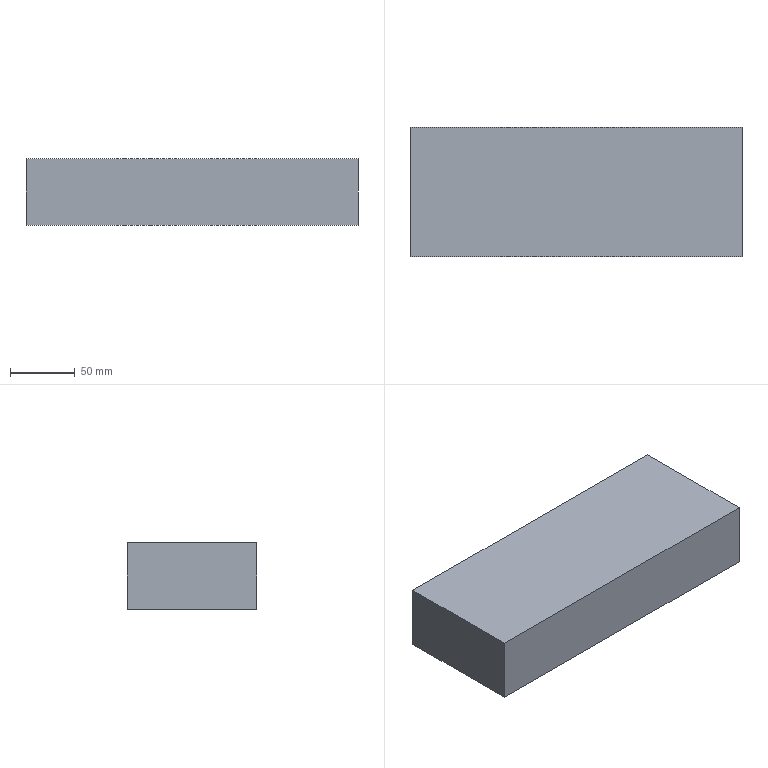Part | SolidWorks | features Extrusion 1, HoleWzd 1 | 1 solid | 22 faces | box 256 x 100 x 51 mm | volume 1305448 mm3 | cylinder 8 | cone 8 | plane 6 | commonest cylinder face diameters 2.5 x8
STEP:
#1=CARTESIAN_POINT('',(-123.,42.5,-18.75));
#2=VERTEX_POINT('',#1);
#3=CARTESIAN_POINT('',(-123.,42.5,-16.25));
#4=VERTEX_POINT('',#3);
#5=CARTESIAN_POINT('',(-123.,42.5,-17.5));
#6=DIRECTION('',(0.,1.,0.));
#7=DIRECTION('',(0.,0.,1.));
#8=AXIS2_PLACEMENT_3D('',#5,#6,#7);
#9=CIRCLE('',#8,1.25);
#10=EDGE_CURVE('',#2,#4,#9,.T.);
#11=ORIENTED_EDGE('',*,*,#10,.F.);
#12=CARTESIAN_POINT('',(-123.,50.,-18.75));
#13=VERTEX_POINT('',#12);
#14=CARTESIAN_POINT('',(-123.,50.,-18.75));
#15=DIRECTION('',(0.,1.,0.));
#16=VECTOR('',#15,1000.);
#17=LINE('',#14,#16);
#18=EDGE_CURVE('',#2,#13,#17,.T.);
#19=ORIENTED_EDGE('',*,*,#18,.T.);
#20=CARTESIAN_POINT('',(-123.,50.,-16.25));
#21=VERTEX_POINT('',#20);
#22=CARTESIAN_POINT('',(-123.,50.,-17.5));
#23=DIRECTION('',(0.,1.,0.));
#24=DIRECTION('',(0.,0.,1.));
#25=AXIS2_PLACEMENT_3D('',#22,#23,#24);
#26=CIRCLE('',#25,1.25);
#27=EDGE_CURVE('',#13,#21,#26,.T.);
#28=ORIENTED_EDGE('',*,*,#27,.T.);
#29=CARTESIAN_POINT('',(-123.,50.,-16.25));
#30=DIRECTION('',(0.,1.,0.));
#31=VECTOR('',#30,1000.);
#32=LINE('',#29,#31);
#33=EDGE_CURVE('',#4,#21,#32,.T.);
#34=ORIENTED_EDGE('',*,*,#33,.F.);
#35=EDGE_LOOP('',(#11,#19,#28,#34));
#36=FACE_OUTER_BOUND('',#35,.T.);
#37=CARTESIAN_POINT('',(-123.,50.,-17.5));
#38=DIRECTION('',(0.,1.,0.));
#39=DIRECTION('',(0.,0.,1.));
#40=AXIS2_PLACEMENT_3D('',#37,#38,#39);
#41=CYLINDRICAL_SURFACE('',#40,1.25);
#42=ADVANCED_FACE('',(#36),#41,.F.);
#43=CARTESIAN_POINT('',(-123.,41.749,-17.5));
#44=VERTEX_POINT('',#43);
#45=CARTESIAN_POINT('',(-123.,42.5,-16.25));
#46=DIRECTION('',(0.,0.515,0.8572));
#47=VECTOR('',#46,1000.);
#48=LINE('',#45,#47);
#49=EDGE_CURVE('',#44,#4,#48,.T.);
#50=ORIENTED_EDGE('',*,*,#49,.F.);
#51=CARTESIAN_POINT('',(-123.,42.5,-18.75));
#52=DIRECTION('',(0.,0.515,-0.8572));
#53=VECTOR('',#52,1000.);
#54=LINE('',#51,#53);
#55=EDGE_CURVE('',#44,#2,#54,.T.);
#56=ORIENTED_EDGE('',*,*,#55,.T.);
#57=ORIENTED_EDGE('',*,*,#10,.T.);
#58=EDGE_LOOP('',(#50,#56,#57));
#59=FACE_OUTER_BOUND('',#58,.T.);
#60=CARTESIAN_POINT('',(-123.,42.5,-17.5));
#61=DIRECTION('',(0.,1.,0.));
#62=DIRECTION('',(0.,0.,1.));
#63=AXIS2_PLACEMENT_3D('',#60,#61,#62);
#64=CONICAL_SURFACE('',#63,1.25,1.03);
#65=ADVANCED_FACE('',(#59),#64,.F.);
#66=CARTESIAN_POINT('',(-123.,42.5,19.25));
#67=VERTEX_POINT('',#66);
#68=CARTESIAN_POINT('',(-123.,42.5,21.75));
#69=VERTEX_POINT('',#68);
#70=CARTESIAN_POINT('',(-123.,42.5,20.5));
#71=DIRECTION('',(0.,1.,0.));
#72=DIRECTION('',(0.,0.,1.));
#73=AXIS2_PLACEMENT_3D('',#70,#71,#72);
#74=CIRCLE('',#73,1.25);
#75=EDGE_CURVE('',#67,#69,#74,.T.);
#76=ORIENTED_EDGE('',*,*,#75,.F.);
#77=CARTESIAN_POINT('',(-123.,50.,19.25));
#78=VERTEX_POINT('',#77);
#79=CARTESIAN_POINT('',(-123.,50.,19.25));
#80=DIRECTION('',(0.,1.,0.));
#81=VECTOR('',#80,1000.);
#82=LINE('',#79,#81);
#83=EDGE_CURVE('',#67,#78,#82,.T.);
#84=ORIENTED_EDGE('',*,*,#83,.T.);
#85=CARTESIAN_POINT('',(-123.,50.,21.75));
#86=VERTEX_POINT('',#85);
#87=CARTESIAN_POINT('',(-123.,50.,20.5));
#88=DIRECTION('',(0.,1.,0.));
#89=DIRECTION('',(0.,0.,1.));
#90=AXIS2_PLACEMENT_3D('',#87,#88,#89);
#91=CIRCLE('',#90,1.25);
#92=EDGE_CURVE('',#78,#86,#91,.T.);
#93=ORIENTED_EDGE('',*,*,#92,.T.);
#94=CARTESIAN_POINT('',(-123.,50.,21.75));
#95=DIRECTION('',(0.,1.,0.));
#96=VECTOR('',#95,1000.);
#97=LINE('',#94,#96);
#98=EDGE_CURVE('',#69,#86,#97,.T.);
#99=ORIENTED_EDGE('',*,*,#98,.F.);
#100=EDGE_LOOP('',(#76,#84,#93,#99));
#101=FACE_OUTER_BOUND('',#100,.T.);
#102=CARTESIAN_POINT('',(-123.,50.,20.5));
#103=DIRECTION('',(0.,1.,0.));
#104=DIRECTION('',(0.,0.,1.));
#105=AXIS2_PLACEMENT_3D('',#102,#103,#104);
#106=CYLINDRICAL_SURFACE('',#105,1.25);
#107=ADVANCED_FACE('',(#101),#106,.F.);
#108=CARTESIAN_POINT('',(-123.,41.749,20.5));
#109=VERTEX_POINT('',#108);
#110=CARTESIAN_POINT('',(-123.,42.5,21.75));
#111=DIRECTION('',(0.,0.515,0.8572));
#112=VECTOR('',#111,1000.);
#113=LINE('',#110,#112);
#114=EDGE_CURVE('',#109,#69,#113,.T.);
#115=ORIENTED_EDGE('',*,*,#114,.F.);
#116=CARTESIAN_POINT('',(-123.,42.5,19.25));
#117=DIRECTION('',(0.,0.515,-0.8572));
#118=VECTOR('',#117,1000.);
#119=LINE('',#116,#118);
#120=EDGE_CURVE('',#109,#67,#119,.T.);
#121=ORIENTED_EDGE('',*,*,#120,.T.);
#122=ORIENTED_EDGE('',*,*,#75,.T.);
#123=EDGE_LOOP('',(#115,#121,#122));
#124=FACE_OUTER_BOUND('',#123,.T.);
#125=CARTESIAN_POINT('',(-123.,42.5,20.5));
#126=DIRECTION('',(0.,1.,0.));
#127=DIRECTION('',(0.,0.,1.));
#128=AXIS2_PLACEMENT_3D('',#125,#126,#127);
#129=CONICAL_SURFACE('',#128,1.25,1.03);
#130=ADVANCED_FACE('',(#124),#129,.F.);
#131=CARTESIAN_POINT('',(123.,42.5,-18.75));
#132=VERTEX_POINT('',#131);
#133=CARTESIAN_POINT('',(123.,42.5,-16.25));
#134=VERTEX_POINT('',#133);
#135=CARTESIAN_POINT('',(123.,42.5,-17.5));
#136=DIRECTION('',(0.,1.,0.));
#137=DIRECTION('',(0.,0.,1.));
#138=AXIS2_PLACEMENT_3D('',#135,#136,#137);
#139=CIRCLE('',#138,1.25);
#140=EDGE_CURVE('',#132,#134,#139,.T.);
#141=ORIENTED_EDGE('',*,*,#140,.F.);
#142=CARTESIAN_POINT('',(123.,50.,-18.75));
#143=VERTEX_POINT('',#142);
#144=CARTESIAN_POINT('',(123.,50.,-18.75));
#145=DIRECTION('',(0.,1.,0.));
#146=VECTOR('',#145,1000.);
#147=LINE('',#144,#146);
#148=EDGE_CURVE('',#132,#143,#147,.T.);
#149=ORIENTED_EDGE('',*,*,#148,.T.);
#150=CARTESIAN_POINT('',(123.,50.,-16.25));
#151=VERTEX_POINT('',#150);
#152=CARTESIAN_POINT('',(123.,50.,-17.5));
#153=DIRECTION('',(0.,1.,0.));
#154=DIRECTION('',(0.,0.,1.));
#155=AXIS2_PLACEMENT_3D('',#152,#153,#154);
#156=CIRCLE('',#155,1.25);
#157=EDGE_CURVE('',#143,#151,#156,.T.);
#158=ORIENTED_EDGE('',*,*,#157,.T.);
#159=CARTESIAN_POINT('',(123.,50.,-16.25));
#160=DIRECTION('',(0.,1.,0.));
#161=VECTOR('',#160,1000.);
#162=LINE('',#159,#161);
#163=EDGE_CURVE('',#134,#151,#162,.T.);
#164=ORIENTED_EDGE('',*,*,#163,.F.);
#165=EDGE_LOOP('',(#141,#149,#158,#164));
#166=FACE_OUTER_BOUND('',#165,.T.);
#167=CARTESIAN_POINT('',(123.,50.,-17.5));
#168=DIRECTION('',(0.,1.,0.));
#169=DIRECTION('',(0.,0.,1.));
#170=AXIS2_PLACEMENT_3D('',#167,#168,#169);
#171=CYLINDRICAL_SURFACE('',#170,1.25);
#172=ADVANCED_FACE('',(#166),#171,.F.);
#173=CARTESIAN_POINT('',(123.,41.749,-17.5));
#174=VERTEX_POINT('',#173);
#175=CARTESIAN_POINT('',(123.,42.5,-16.25));
#176=DIRECTION('',(0.,0.515,0.8572));
#177=VECTOR('',#176,1000.);
#178=LINE('',#175,#177);
#179=EDGE_CURVE('',#174,#134,#178,.T.);
#180=ORIENTED_EDGE('',*,*,#179,.F.);
#181=CARTESIAN_POINT('',(123.,42.5,-18.75));
#182=DIRECTION('',(0.,0.515,-0.8572));
#183=VECTOR('',#182,1000.);
#184=LINE('',#181,#183);
#185=EDGE_CURVE('',#174,#132,#184,.T.);
#186=ORIENTED_EDGE('',*,*,#185,.T.);
#187=ORIENTED_EDGE('',*,*,#140,.T.);
#188=EDGE_LOOP('',(#180,#186,#187));
#189=FACE_OUTER_BOUND('',#188,.T.);
#190=CARTESIAN_POINT('',(123.,42.5,-17.5));
#191=DIRECTION('',(0.,1.,0.));
#192=DIRECTION('',(0.,0.,1.));
#193=AXIS2_PLACEMENT_3D('',#190,#191,#192);
#194=CONICAL_SURFACE('',#193,1.25,1.03);
#195=ADVANCED_FACE('',(#189),#194,.F.);
#196=CARTESIAN_POINT('',(123.,42.5,19.25));
#197=VERTEX_POINT('',#196);
#198=CARTESIAN_POINT('',(123.,42.5,21.75));
#199=VERTEX_POINT('',#198);
#200=CARTESIAN_POINT('',(123.,42.5,20.5));
#201=DIRECTION('',(0.,1.,0.));
#202=DIRECTION('',(0.,0.,1.));
#203=AXIS2_PLACEMENT_3D('',#200,#201,#202);
#204=CIRCLE('',#203,1.25);
#205=EDGE_CURVE('',#197,#199,#204,.T.);
#206=ORIENTED_EDGE('',*,*,#205,.F.);
#207=CARTESIAN_POINT('',(123.,50.,19.25));
#208=VERTEX_POINT('',#207);
#209=CARTESIAN_POINT('',(123.,50.,19.25));
#210=DIRECTION('',(0.,1.,0.));
#211=VECTOR('',#210,1000.);
#212=LINE('',#209,#211);
#213=EDGE_CURVE('',#197,#208,#212,.T.);
#214=ORIENTED_EDGE('',*,*,#213,.T.);
#215=CARTESIAN_POINT('',(123.,50.,21.75));
#216=VERTEX_POINT('',#215);
#217=CARTESIAN_POINT('',(123.,50.,20.5));
#218=DIRECTION('',(0.,1.,0.));
#219=DIRECTION('',(0.,0.,1.));
#220=AXIS2_PLACEMENT_3D('',#217,#218,#219);
#221=CIRCLE('',#220,1.25);
#222=EDGE_CURVE('',#208,#216,#221,.T.);
#223=ORIENTED_EDGE('',*,*,#222,.T.);
#224=CARTESIAN_POINT('',(123.,50.,21.75));
#225=DIRECTION('',(0.,1.,0.));
#226=VECTOR('',#225,1000.);
#227=LINE('',#224,#226);
#228=EDGE_CURVE('',#199,#216,#227,.T.);
#229=ORIENTED_EDGE('',*,*,#228,.F.);
#230=EDGE_LOOP('',(#206,#214,#223,#229));
#231=FACE_OUTER_BOUND('',#230,.T.);
#232=CARTESIAN_POINT('',(123.,50.,20.5));
#233=DIRECTION('',(0.,1.,0.));
#234=DIRECTION('',(0.,0.,1.));
#235=AXIS2_PLACEMENT_3D('',#232,#233,#234);
#236=CYLINDRICAL_SURFACE('',#235,1.25);
#237=ADVANCED_FACE('',(#231),#236,.F.);
#238=CARTESIAN_POINT('',(123.,41.749,20.5));
#239=VERTEX_POINT('',#238);
#240=CARTESIAN_POINT('',(123.,42.5,21.75));
#241=DIRECTION('',(0.,0.515,0.8572));
#242=VECTOR('',#241,1000.);
#243=LINE('',#240,#242);
#244=EDGE_CURVE('',#239,#199,#243,.T.);
#245=ORIENTED_EDGE('',*,*,#244,.F.);
#246=CARTESIAN_POINT('',(123.,42.5,19.25));
#247=DIRECTION('',(0.,0.515,-0.8572));
#248=VECTOR('',#247,1000.);
#249=LINE('',#246,#248);
#250=EDGE_CURVE('',#239,#197,#249,.T.);
#251=ORIENTED_EDGE('',*,*,#250,.T.);
#252=ORIENTED_EDGE('',*,*,#205,.T.);
#253=EDGE_LOOP('',(#245,#251,#252));
#254=FACE_OUTER_BOUND('',#253,.T.);
#255=CARTESIAN_POINT('',(123.,42.5,20.5));
#256=DIRECTION('',(0.,1.,0.));
#257=DIRECTION('',(0.,0.,1.));
#258=AXIS2_PLACEMENT_3D('',#255,#256,#257);
#259=CONICAL_SURFACE('',#258,1.25,1.03);
#260=ADVANCED_FACE('',(#254),#259,.F.);
#261=CARTESIAN_POINT('',(128.,-50.,-25.5));
#262=VERTEX_POINT('',#261);
#263=CARTESIAN_POINT('',(128.,50.,-25.5));
#264=VERTEX_POINT('',#263);
#265=CARTESIAN_POINT('',(128.,-50.,-25.5));
#266=DIRECTION('',(0.,1.,0.));
#267=VECTOR('',#266,1000.);
#268=LINE('',#265,#267);
#269=EDGE_CURVE('',#262,#264,#268,.T.);
#270=ORIENTED_EDGE('',*,*,#269,.T.);
#271=CARTESIAN_POINT('',(128.,50.,25.5));
#272=VERTEX_POINT('',#271);
#273=CARTESIAN_POINT('',(128.,50.,25.5));
#274=DIRECTION('',(0.,0.,-1.));
#275=VECTOR('',#274,1000.);
#276=LINE('',#273,#275);
#277=EDGE_CURVE('',#272,#264,#276,.T.);
#278=ORIENTED_EDGE('',*,*,#277,.F.);
#279=CARTESIAN_POINT('',(128.,-50.,25.5));
#280=VERTEX_POINT('',#279);
#281=CARTESIAN_POINT('',(128.,-50.,25.5));
#282=DIRECTION('',(0.,1.,0.));
#283=VECTOR('',#282,1000.);
#284=LINE('',#281,#283);
#285=EDGE_CURVE('',#280,#272,#284,.T.);
#286=ORIENTED_EDGE('',*,*,#285,.F.);
#287=CARTESIAN_POINT('',(128.,-50.,25.5));
#288=DIRECTION('',(0.,0.,-1.));
#289=VECTOR('',#288,1000.);
#290=LINE('',#287,#289);
#291=EDGE_CURVE('',#280,#262,#290,.T.);
#292=ORIENTED_EDGE('',*,*,#291,.T.);
#293=EDGE_LOOP('',(#270,#278,#286,#292));
#294=FACE_OUTER_BOUND('',#293,.T.);
#295=CARTESIAN_POINT('',(128.,-50.,25.5));
#296=DIRECTION('',(-1.,0.,0.));
#297=DIRECTION('',(0.,0.,1.));
#298=AXIS2_PLACEMENT_3D('',#295,#296,#297);
#299=PLANE('',#298);
#300=ADVANCED_FACE('',(#294),#299,.F.);
#301=CARTESIAN_POINT('',(-123.,50.,-17.5));
#302=DIRECTION('',(0.,1.,0.));
#303=DIRECTION('',(0.,0.,1.));
#304=AXIS2_PLACEMENT_3D('',#301,#302,#303);
#305=CIRCLE('',#304,1.25);
#306=EDGE_CURVE('',#21,#13,#305,.T.);
#307=ORIENTED_EDGE('',*,*,#306,.F.);
#308=ORIENTED_EDGE('',*,*,#27,.F.);
#309=EDGE_LOOP('',(#307,#308));
#310=FACE_BOUND('',#309,.T.);
#311=CARTESIAN_POINT('',(-123.,50.,20.5));
#312=DIRECTION('',(0.,1.,0.));
#313=DIRECTION('',(0.,0.,1.));
#314=AXIS2_PLACEMENT_3D('',#311,#312,#313);
#315=CIRCLE('',#314,1.25);
#316=EDGE_CURVE('',#86,#78,#315,.T.);
#317=ORIENTED_EDGE('',*,*,#316,.F.);
#318=ORIENTED_EDGE('',*,*,#92,.F.);
#319=EDGE_LOOP('',(#317,#318));
#320=FACE_BOUND('',#319,.T.);
#321=CARTESIAN_POINT('',(123.,50.,-17.5));
#322=DIRECTION('',(0.,1.,0.));
#323=DIRECTION('',(0.,0.,1.));
#324=AXIS2_PLACEMENT_3D('',#321,#322,#323);
#325=CIRCLE('',#324,1.25);
#326=EDGE_CURVE('',#151,#143,#325,.T.);
#327=ORIENTED_EDGE('',*,*,#326,.F.);
#328=ORIENTED_EDGE('',*,*,#157,.F.);
#329=EDGE_LOOP('',(#327,#328));
#330=FACE_BOUND('',#329,.T.);
#331=CARTESIAN_POINT('',(123.,50.,20.5));
#332=DIRECTION('',(0.,1.,0.));
#333=DIRECTION('',(0.,0.,1.));
#334=AXIS2_PLACEMENT_3D('',#331,#332,#333);
#335=CIRCLE('',#334,1.25);
#336=EDGE_CURVE('',#216,#208,#335,.T.);
#337=ORIENTED_EDGE('',*,*,#336,.F.);
#338=ORIENTED_EDGE('',*,*,#222,.F.);
#339=EDGE_LOOP('',(#337,#338));
#340=FACE_BOUND('',#339,.T.);
#341=CARTESIAN_POINT('',(-128.,50.,-25.5));
#342=VERTEX_POINT('',#341);
#343=CARTESIAN_POINT('',(-128.,50.,-25.5));
#344=DIRECTION('',(-1.,0.,0.));
#345=VECTOR('',#344,1000.);
#346=LINE('',#343,#345);
#347=EDGE_CURVE('',#264,#342,#346,.T.);
#348=ORIENTED_EDGE('',*,*,#347,.T.);
#349=CARTESIAN_POINT('',(-128.,50.,25.5));
#350=VERTEX_POINT('',#349);
#351=CARTESIAN_POINT('',(-128.,50.,25.5));
#352=DIRECTION('',(0.,0.,-1.));
#353=VECTOR('',#352,1000.);
#354=LINE('',#351,#353);
#355=EDGE_CURVE('',#350,#342,#354,.T.);
#356=ORIENTED_EDGE('',*,*,#355,.F.);
#357=CARTESIAN_POINT('',(-128.,50.,25.5));
#358=DIRECTION('',(-1.,0.,0.));
#359=VECTOR('',#358,1000.);
#360=LINE('',#357,#359);
#361=EDGE_CURVE('',#272,#350,#360,.T.);
#362=ORIENTED_EDGE('',*,*,#361,.F.);
#363=ORIENTED_EDGE('',*,*,#277,.T.);
#364=EDGE_LOOP('',(#348,#356,#362,#363));
#365=FACE_OUTER_BOUND('',#364,.T.);
#366=CARTESIAN_POINT('',(-128.,50.,25.5));
#367=DIRECTION('',(0.,-1.,0.));
#368=DIRECTION('',(0.,0.,-1.));
#369=AXIS2_PLACEMENT_3D('',#366,#367,#368);
#370=PLANE('',#369);
#371=ADVANCED_FACE('',(#310,#320,#330,#340,#365),#370,.F.);
#372=CARTESIAN_POINT('',(-128.,-50.,-25.5));
#373=VERTEX_POINT('',#372);
#374=CARTESIAN_POINT('',(-128.,-50.,-25.5));
#375=DIRECTION('',(0.,-1.,0.));
#376=VECTOR('',#375,1000.);
#377=LINE('',#374,#376);
#378=EDGE_CURVE('',#342,#373,#377,.T.);
#379=ORIENTED_EDGE('',*,*,#378,.T.);
#380=CARTESIAN_POINT('',(-128.,-50.,25.5));
#381=VERTEX_POINT('',#380);
#382=CARTESIAN_POINT('',(-128.,-50.,25.5));
#383=DIRECTION('',(0.,0.,-1.));
#384=VECTOR('',#383,1000.);
#385=LINE('',#382,#384);
#386=EDGE_CURVE('',#381,#373,#385,.T.);
#387=ORIENTED_EDGE('',*,*,#386,.F.);
#388=CARTESIAN_POINT('',(-128.,-50.,25.5));
#389=DIRECTION('',(0.,-1.,0.));
#390=VECTOR('',#389,1000.);
#391=LINE('',#388,#390);
#392=EDGE_CURVE('',#350,#381,#391,.T.);
#393=ORIENTED_EDGE('',*,*,#392,.F.);
#394=ORIENTED_EDGE('',*,*,#355,.T.);
#395=EDGE_LOOP('',(#379,#387,#393,#394));
#396=FACE_OUTER_BOUND('',#395,.T.);
#397=CARTESIAN_POINT('',(-128.,-50.,25.5));
#398=DIRECTION('',(1.,0.,0.));
#399=DIRECTION('',(0.,0.,-1.));
#400=AXIS2_PLACEMENT_3D('',#397,#398,#399);
#401=PLANE('',#400);
#402=ADVANCED_FACE('',(#396),#401,.F.);
#403=CARTESIAN_POINT('',(-128.,-50.,-25.5));
#404=DIRECTION('',(1.,0.,0.));
#405=VECTOR('',#404,1000.);
#406=LINE('',#403,#405);
#407=EDGE_CURVE('',#373,#262,#406,.T.);
#408=ORIENTED_EDGE('',*,*,#407,.T.);
#409=ORIENTED_EDGE('',*,*,#291,.F.);
#410=CARTESIAN_POINT('',(-128.,-50.,25.5));
#411=DIRECTION('',(1.,0.,0.));
#412=VECTOR('',#411,1000.);
#413=LINE('',#410,#412);
#414=EDGE_CURVE('',#381,#280,#413,.T.);
#415=ORIENTED_EDGE('',*,*,#414,.F.);
#416=ORIENTED_EDGE('',*,*,#386,.T.);
#417=EDGE_LOOP('',(#408,#409,#415,#416));
#418=FACE_OUTER_BOUND('',#417,.T.);
#419=CARTESIAN_POINT('',(-128.,-50.,25.5));
#420=DIRECTION('',(0.,1.,0.));
#421=DIRECTION('',(0.,0.,1.));
#422=AXIS2_PLACEMENT_3D('',#419,#420,#421);
#423=PLANE('',#422);
#424=ADVANCED_FACE('',(#418),#423,.F.);
#425=ORIENTED_EDGE('',*,*,#285,.T.);
#426=ORIENTED_EDGE('',*,*,#361,.T.);
#427=ORIENTED_EDGE('',*,*,#392,.T.);
#428=ORIENTED_EDGE('',*,*,#414,.T.);
#429=EDGE_LOOP('',(#425,#426,#427,#428));
#430=FACE_OUTER_BOUND('',#429,.T.);
#431=CARTESIAN_POINT('',(0.,0.,25.5));
#432=DIRECTION('',(0.,0.,-1.));
#433=DIRECTION('',(-1.,0.,0.));
#434=AXIS2_PLACEMENT_3D('',#431,#432,#433);
#435=PLANE('',#434);
#436=ADVANCED_FACE('',(#430),#435,.F.);
#437=ORIENTED_EDGE('',*,*,#269,.F.);
#438=ORIENTED_EDGE('',*,*,#407,.F.);
#439=ORIENTED_EDGE('',*,*,#378,.F.);
#440=ORIENTED_EDGE('',*,*,#347,.F.);
#441=EDGE_LOOP('',(#437,#438,#439,#440));
#442=FACE_OUTER_BOUND('',#441,.T.);
#443=CARTESIAN_POINT('',(0.,0.,-25.5));
#444=DIRECTION('',(0.,0.,-1.));
#445=DIRECTION('',(-1.,0.,0.));
#446=AXIS2_PLACEMENT_3D('',#443,#444,#445);
#447=PLANE('',#446);
#448=ADVANCED_FACE('',(#442),#447,.T.);
#449=ORIENTED_EDGE('',*,*,#250,.F.);
#450=ORIENTED_EDGE('',*,*,#244,.T.);
#451=CARTESIAN_POINT('',(123.,42.5,20.5));
#452=DIRECTION('',(0.,1.,0.));
#453=DIRECTION('',(0.,0.,1.));
#454=AXIS2_PLACEMENT_3D('',#451,#452,#453);
#455=CIRCLE('',#454,1.25);
#456=EDGE_CURVE('',#199,#197,#455,.T.);
#457=ORIENTED_EDGE('',*,*,#456,.T.);
#458=EDGE_LOOP('',(#449,#450,#457));
#459=FACE_OUTER_BOUND('',#458,.T.);
#460=CARTESIAN_POINT('',(123.,42.5,20.5));
#461=DIRECTION('',(0.,1.,0.));
#462=DIRECTION('',(0.,0.,1.));
#463=AXIS2_PLACEMENT_3D('',#460,#461,#462);
#464=CONICAL_SURFACE('',#463,1.25,1.03);
#465=ADVANCED_FACE('',(#459),#464,.F.);
#466=ORIENTED_EDGE('',*,*,#213,.F.);
#467=ORIENTED_EDGE('',*,*,#456,.F.);
#468=ORIENTED_EDGE('',*,*,#228,.T.);
#469=ORIENTED_EDGE('',*,*,#336,.T.);
#470=EDGE_LOOP('',(#466,#467,#468,#469));
#471=FACE_OUTER_BOUND('',#470,.T.);
#472=CARTESIAN_POINT('',(123.,50.,20.5));
#473=DIRECTION('',(0.,1.,0.));
#474=DIRECTION('',(0.,0.,1.));
#475=AXIS2_PLACEMENT_3D('',#472,#473,#474);
#476=CYLINDRICAL_SURFACE('',#475,1.25);
#477=ADVANCED_FACE('',(#471),#476,.F.);
#478=ORIENTED_EDGE('',*,*,#185,.F.);
#479=ORIENTED_EDGE('',*,*,#179,.T.);
#480=CARTESIAN_POINT('',(123.,42.5,-17.5));
#481=DIRECTION('',(0.,1.,0.));
#482=DIRECTION('',(0.,0.,1.));
#483=AXIS2_PLACEMENT_3D('',#480,#481,#482);
#484=CIRCLE('',#483,1.25);
#485=EDGE_CURVE('',#134,#132,#484,.T.);
#486=ORIENTED_EDGE('',*,*,#485,.T.);
#487=EDGE_LOOP('',(#478,#479,#486));
#488=FACE_OUTER_BOUND('',#487,.T.);
#489=CARTESIAN_POINT('',(123.,42.5,-17.5));
#490=DIRECTION('',(0.,1.,0.));
#491=DIRECTION('',(0.,0.,1.));
#492=AXIS2_PLACEMENT_3D('',#489,#490,#491);
#493=CONICAL_SURFACE('',#492,1.25,1.03);
#494=ADVANCED_FACE('',(#488),#493,.F.);
#495=ORIENTED_EDGE('',*,*,#148,.F.);
#496=ORIENTED_EDGE('',*,*,#485,.F.);
#497=ORIENTED_EDGE('',*,*,#163,.T.);
#498=ORIENTED_EDGE('',*,*,#326,.T.);
#499=EDGE_LOOP('',(#495,#496,#497,#498));
#500=FACE_OUTER_BOUND('',#499,.T.);
#501=CARTESIAN_POINT('',(123.,50.,-17.5));
#502=DIRECTION('',(0.,1.,0.));
#503=DIRECTION('',(0.,0.,1.));
#504=AXIS2_PLACEMENT_3D('',#501,#502,#503);
#505=CYLINDRICAL_SURFACE('',#504,1.25);
#506=ADVANCED_FACE('',(#500),#505,.F.);
#507=ORIENTED_EDGE('',*,*,#120,.F.);
#508=ORIENTED_EDGE('',*,*,#114,.T.);
#509=CARTESIAN_POINT('',(-123.,42.5,20.5));
#510=DIRECTION('',(0.,1.,0.));
#511=DIRECTION('',(0.,0.,1.));
#512=AXIS2_PLACEMENT_3D('',#509,#510,#511);
#513=CIRCLE('',#512,1.25);
#514=EDGE_CURVE('',#69,#67,#513,.T.);
#515=ORIENTED_EDGE('',*,*,#514,.T.);
#516=EDGE_LOOP('',(#507,#508,#515));
#517=FACE_OUTER_BOUND('',#516,.T.);
#518=CARTESIAN_POINT('',(-123.,42.5,20.5));
#519=DIRECTION('',(0.,1.,0.));
#520=DIRECTION('',(0.,0.,1.));
#521=AXIS2_PLACEMENT_3D('',#518,#519,#520);
#522=CONICAL_SURFACE('',#521,1.25,1.03);
#523=ADVANCED_FACE('',(#517),#522,.F.);
#524=ORIENTED_EDGE('',*,*,#83,.F.);
#525=ORIENTED_EDGE('',*,*,#514,.F.);
#526=ORIENTED_EDGE('',*,*,#98,.T.);
#527=ORIENTED_EDGE('',*,*,#316,.T.);
#528=EDGE_LOOP('',(#524,#525,#526,#527));
#529=FACE_OUTER_BOUND('',#528,.T.);
#530=CARTESIAN_POINT('',(-123.,50.,20.5));
#531=DIRECTION('',(0.,1.,0.));
#532=DIRECTION('',(0.,0.,1.));
#533=AXIS2_PLACEMENT_3D('',#530,#531,#532);
#534=CYLINDRICAL_SURFACE('',#533,1.25);
#535=ADVANCED_FACE('',(#529),#534,.F.);
#536=ORIENTED_EDGE('',*,*,#55,.F.);
#537=ORIENTED_EDGE('',*,*,#49,.T.);
#538=CARTESIAN_POINT('',(-123.,42.5,-17.5));
#539=DIRECTION('',(0.,1.,0.));
#540=DIRECTION('',(0.,0.,1.));
#541=AXIS2_PLACEMENT_3D('',#538,#539,#540);
#542=CIRCLE('',#541,1.25);
#543=EDGE_CURVE('',#4,#2,#542,.T.);
#544=ORIENTED_EDGE('',*,*,#543,.T.);
#545=EDGE_LOOP('',(#536,#537,#544));
#546=FACE_OUTER_BOUND('',#545,.T.);
#547=CARTESIAN_POINT('',(-123.,42.5,-17.5));
#548=DIRECTION('',(0.,1.,0.));
#549=DIRECTION('',(0.,0.,1.));
#550=AXIS2_PLACEMENT_3D('',#547,#548,#549);
#551=CONICAL_SURFACE('',#550,1.25,1.03);
#552=ADVANCED_FACE('',(#546),#551,.F.);
#553=ORIENTED_EDGE('',*,*,#18,.F.);
#554=ORIENTED_EDGE('',*,*,#543,.F.);
#555=ORIENTED_EDGE('',*,*,#33,.T.);
#556=ORIENTED_EDGE('',*,*,#306,.T.);
#557=EDGE_LOOP('',(#553,#554,#555,#556));
#558=FACE_OUTER_BOUND('',#557,.T.);
#559=CARTESIAN_POINT('',(-123.,50.,-17.5));
#560=DIRECTION('',(0.,1.,0.));
#561=DIRECTION('',(0.,0.,1.));
#562=AXIS2_PLACEMENT_3D('',#559,#560,#561);
#563=CYLINDRICAL_SURFACE('',#562,1.25);
#564=ADVANCED_FACE('',(#558),#563,.F.);
#565=CLOSED_SHELL('',(#42,#65,#107,#130,#172,#195,#237,#260,#300,#371,#402,#424,#436,#448,#465,#477,#494,#506,#523,#535,#552,#564));
#566=MANIFOLD_SOLID_BREP('',#565);
#567=CARTESIAN_POINT('',(0.,0.,0.));
#568=DIRECTION('',(0.,0.,1.));
#569=DIRECTION('',(1.,0.,0.));
#570=AXIS2_PLACEMENT_3D('',#567,#568,#569);
#571=(LENGTH_UNIT()NAMED_UNIT(*)SI_UNIT(.MILLI.,.METRE.));
#572=UNCERTAINTY_MEASURE_WITH_UNIT(LENGTH_MEASURE(0.00001),#571,'','');
#573=(NAMED_UNIT(*)PLANE_ANGLE_UNIT()SI_UNIT($,.RADIAN.));
#574=(NAMED_UNIT(*)SI_UNIT($,.STERADIAN.)SOLID_ANGLE_UNIT());
#575=(GEOMETRIC_REPRESENTATION_CONTEXT(3)GLOBAL_UNCERTAINTY_ASSIGNED_CONTEXT((#572))GLOBAL_UNIT_ASSIGNED_CONTEXT((#571,#573,#574))REPRESENTATION_CONTEXT('',''));
#576=ADVANCED_BREP_SHAPE_REPRESENTATION('',(#566,#570),#575);